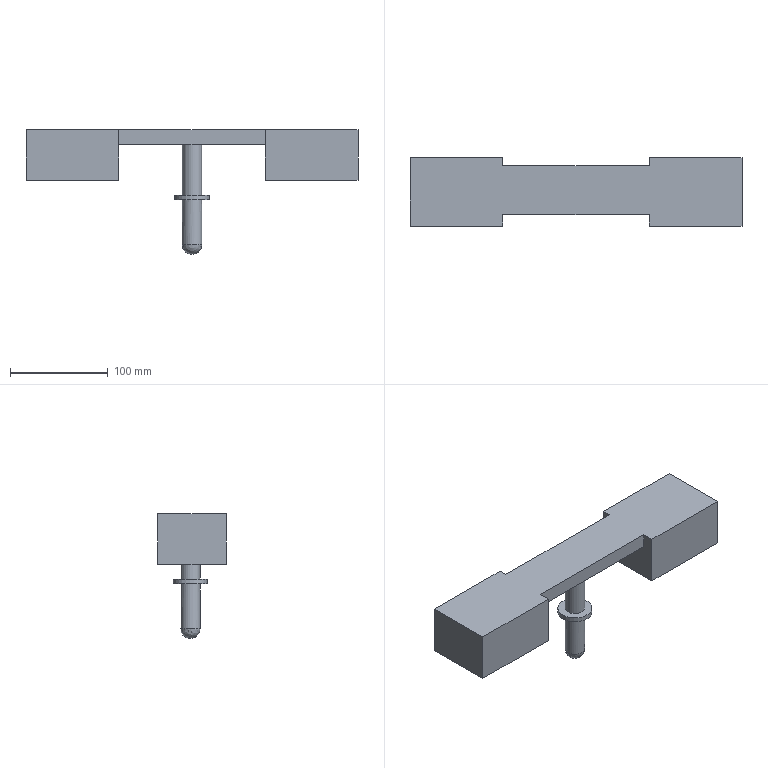Part | STEP file | tieqiantou | 1 solid | 20 faces | box 340 x 70 x 128 mm | volume 841793 mm3 | plane 16 | cylinder 3 | sphere 1 | commonest cylinder face diameters 20 x2 35 x1
STEP:
#1=CARTESIAN_POINT('',(0.,0.,0.));
#2=DIRECTION('',(0.,0.,1.));
#3=DIRECTION('',(1.,0.,0.));
#4=AXIS2_PLACEMENT_3D('',#1,#2,#3);
#5=CARTESIAN_POINT('',(-10.,0.,113.));
#6=VERTEX_POINT('',#5);
#7=CARTESIAN_POINT('',(10.,0.,113.));
#8=VERTEX_POINT('',#7);
#9=CARTESIAN_POINT('',(0.,0.,113.));
#10=DIRECTION('',(0.,0.,1.));
#11=DIRECTION('',(1.,0.,0.));
#12=AXIS2_PLACEMENT_3D('',#9,#10,#11);
#13=CIRCLE('',#12,10.);
#14=CARTESIAN_POINT('',(0.,0.,113.));
#15=DIRECTION('',(0.,0.,-1.));
#16=DIRECTION('',(-1.,0.,0.));
#17=AXIS2_PLACEMENT_3D('',#14,#15,#16);
#18=CYLINDRICAL_SURFACE('',#17,10.);
#19=CARTESIAN_POINT('',(9.425,0.));
#20=DIRECTION('',(-1.,0.));
#21=VECTOR('',#20,1.);
#22=LINE('',#19,#21);
#23=(GEOMETRIC_REPRESENTATION_CONTEXT(2)PARAMETRIC_REPRESENTATION_CONTEXT()REPRESENTATION_CONTEXT('',''));
#24=DEFINITIONAL_REPRESENTATION('',(#22),#23);
#25=PCURVE('',#18,#24);
#26=CARTESIAN_POINT('',(0.,0.,113.));
#27=DIRECTION('',(0.,0.,1.));
#28=DIRECTION('',(1.,0.,0.));
#29=AXIS2_PLACEMENT_3D('',#26,#27,#28);
#30=PLANE('',#29);
#31=CARTESIAN_POINT('',(0.,0.));
#32=DIRECTION('',(1.,0.));
#33=AXIS2_PLACEMENT_2D('',#31,#32);
#34=CIRCLE('',#33,10.);
#35=(GEOMETRIC_REPRESENTATION_CONTEXT(2)PARAMETRIC_REPRESENTATION_CONTEXT()REPRESENTATION_CONTEXT('',''));
#36=DEFINITIONAL_REPRESENTATION('',(#34),#35);
#37=PCURVE('',#30,#36);
#38=SURFACE_CURVE('',#13,(#25,#37),.PCURVE_S1.);
#39=EDGE_CURVE('',#6,#8,#38,.T.);
#40=ORIENTED_EDGE('',*,*,#39,.F.);
#41=CARTESIAN_POINT('',(-10.,0.,61.));
#42=VERTEX_POINT('',#41);
#43=CARTESIAN_POINT('',(-10.,0.,113.));
#44=CARTESIAN_POINT('',(-10.,0.,61.));
#45=B_SPLINE_CURVE_WITH_KNOTS('',1,(#43,#44),.UNSPECIFIED.,.F.,.F.,(2,2),(0.,52.),.PIECEWISE_BEZIER_KNOTS.);
#46=CARTESIAN_POINT('',(6.283,0.));
#47=DIRECTION('',(0.,1.));
#48=VECTOR('',#47,1.);
#49=LINE('',#46,#48);
#50=(GEOMETRIC_REPRESENTATION_CONTEXT(2)PARAMETRIC_REPRESENTATION_CONTEXT()REPRESENTATION_CONTEXT('',''));
#51=DEFINITIONAL_REPRESENTATION('',(#49),#50);
#52=PCURVE('',#18,#51);
#53=CARTESIAN_POINT('',(0.,0.));
#54=DIRECTION('',(0.,1.));
#55=VECTOR('',#54,1.);
#56=LINE('',#53,#55);
#57=(GEOMETRIC_REPRESENTATION_CONTEXT(2)PARAMETRIC_REPRESENTATION_CONTEXT()REPRESENTATION_CONTEXT('',''));
#58=DEFINITIONAL_REPRESENTATION('',(#56),#57);
#59=PCURVE('',#18,#58);
#60=SEAM_CURVE('',#45,(#52,#59),.PCURVE_S1.);
#61=EDGE_CURVE('',#6,#42,#60,.T.);
#62=ORIENTED_EDGE('',*,*,#61,.T.);
#63=CARTESIAN_POINT('',(0.,0.,61.));
#64=DIRECTION('',(0.,0.,-1.));
#65=DIRECTION('',(-1.,0.,0.));
#66=AXIS2_PLACEMENT_3D('',#63,#64,#65);
#67=CIRCLE('',#66,10.);
#68=CARTESIAN_POINT('',(0.,52.));
#69=DIRECTION('',(1.,0.));
#70=VECTOR('',#69,1.);
#71=LINE('',#68,#70);
#72=(GEOMETRIC_REPRESENTATION_CONTEXT(2)PARAMETRIC_REPRESENTATION_CONTEXT()REPRESENTATION_CONTEXT('',''));
#73=DEFINITIONAL_REPRESENTATION('',(#71),#72);
#74=PCURVE('',#18,#73);
#75=CARTESIAN_POINT('',(0.,0.,61.));
#76=DIRECTION('',(0.,0.,-1.));
#77=DIRECTION('',(-1.,0.,0.));
#78=AXIS2_PLACEMENT_3D('',#75,#76,#77);
#79=PLANE('',#78);
#80=CARTESIAN_POINT('',(0.,0.));
#81=DIRECTION('',(1.,0.));
#82=AXIS2_PLACEMENT_2D('',#80,#81);
#83=CIRCLE('',#82,10.);
#84=(GEOMETRIC_REPRESENTATION_CONTEXT(2)PARAMETRIC_REPRESENTATION_CONTEXT()REPRESENTATION_CONTEXT('',''));
#85=DEFINITIONAL_REPRESENTATION('',(#83),#84);
#86=PCURVE('',#79,#85);
#87=SURFACE_CURVE('',#67,(#74,#86),.PCURVE_S1.);
#88=EDGE_CURVE('',#42,#42,#87,.T.);
#89=ORIENTED_EDGE('',*,*,#88,.F.);
#90=ORIENTED_EDGE('',*,*,#61,.F.);
#91=CARTESIAN_POINT('',(0.,0.,113.));
#92=DIRECTION('',(0.,0.,1.));
#93=DIRECTION('',(1.,0.,0.));
#94=AXIS2_PLACEMENT_3D('',#91,#92,#93);
#95=CIRCLE('',#94,10.);
#96=CARTESIAN_POINT('',(3.142,0.));
#97=DIRECTION('',(-1.,0.));
#98=VECTOR('',#97,1.);
#99=LINE('',#96,#98);
#100=(GEOMETRIC_REPRESENTATION_CONTEXT(2)PARAMETRIC_REPRESENTATION_CONTEXT()REPRESENTATION_CONTEXT('',''));
#101=DEFINITIONAL_REPRESENTATION('',(#99),#100);
#102=PCURVE('',#18,#101);
#103=CARTESIAN_POINT('',(0.,0.));
#104=DIRECTION('',(1.,0.));
#105=AXIS2_PLACEMENT_2D('',#103,#104);
#106=CIRCLE('',#105,10.);
#107=(GEOMETRIC_REPRESENTATION_CONTEXT(2)PARAMETRIC_REPRESENTATION_CONTEXT()REPRESENTATION_CONTEXT('',''));
#108=DEFINITIONAL_REPRESENTATION('',(#106),#107);
#109=PCURVE('',#30,#108);
#110=SURFACE_CURVE('',#95,(#102,#109),.PCURVE_S1.);
#111=EDGE_CURVE('',#8,#6,#110,.T.);
#112=ORIENTED_EDGE('',*,*,#111,.F.);
#113=EDGE_LOOP('',(#40,#62,#89,#90,#112));
#114=FACE_BOUND('',#113,.T.);
#115=ADVANCED_FACE('',(#114),#18,.T.);
#116=ORIENTED_EDGE('',*,*,#111,.T.);
#117=ORIENTED_EDGE('',*,*,#39,.T.);
#118=EDGE_LOOP('',(#116,#117));
#119=FACE_BOUND('',#118,.T.);
#120=CARTESIAN_POINT('',(75.,-25.,113.));
#121=VERTEX_POINT('',#120);
#122=CARTESIAN_POINT('',(75.,25.,113.));
#123=VERTEX_POINT('',#122);
#124=CARTESIAN_POINT('',(75.,25.,113.));
#125=DIRECTION('',(0.,1.,0.));
#126=VECTOR('',#125,1.);
#127=LINE('',#124,#126);
#128=CARTESIAN_POINT('',(75.,25.));
#129=DIRECTION('',(0.,1.));
#130=VECTOR('',#129,1.);
#131=LINE('',#128,#130);
#132=(GEOMETRIC_REPRESENTATION_CONTEXT(2)PARAMETRIC_REPRESENTATION_CONTEXT()REPRESENTATION_CONTEXT('',''));
#133=DEFINITIONAL_REPRESENTATION('',(#131),#132);
#134=PCURVE('',#30,#133);
#135=CARTESIAN_POINT('',(75.,33.294,76.));
#136=DIRECTION('',(1.,0.,0.));
#137=DIRECTION('',(0.,1.,0.));
#138=AXIS2_PLACEMENT_3D('',#135,#136,#137);
#139=PLANE('',#138);
#140=CARTESIAN_POINT('',(-8.294,37.));
#141=DIRECTION('',(1.,0.));
#142=VECTOR('',#141,1.);
#143=LINE('',#140,#142);
#144=(GEOMETRIC_REPRESENTATION_CONTEXT(2)PARAMETRIC_REPRESENTATION_CONTEXT()REPRESENTATION_CONTEXT('',''));
#145=DEFINITIONAL_REPRESENTATION('',(#143),#144);
#146=PCURVE('',#139,#145);
#147=SURFACE_CURVE('',#127,(#134,#146),.PCURVE_S1.);
#148=EDGE_CURVE('',#121,#123,#147,.T.);
#149=ORIENTED_EDGE('',*,*,#148,.F.);
#150=CARTESIAN_POINT('',(-75.,-25.,113.));
#151=VERTEX_POINT('',#150);
#152=CARTESIAN_POINT('',(-75.,-25.,113.));
#153=DIRECTION('',(1.,0.,0.));
#154=VECTOR('',#153,1.);
#155=LINE('',#152,#154);
#156=CARTESIAN_POINT('',(-75.,-25.));
#157=DIRECTION('',(1.,0.));
#158=VECTOR('',#157,1.);
#159=LINE('',#156,#158);
#160=(GEOMETRIC_REPRESENTATION_CONTEXT(2)PARAMETRIC_REPRESENTATION_CONTEXT()REPRESENTATION_CONTEXT('',''));
#161=DEFINITIONAL_REPRESENTATION('',(#159),#160);
#162=PCURVE('',#30,#161);
#163=CARTESIAN_POINT('',(-75.,-25.,113.));
#164=DIRECTION('',(0.,-1.,0.));
#165=DIRECTION('',(0.,0.,-1.));
#166=AXIS2_PLACEMENT_3D('',#163,#164,#165);
#167=PLANE('',#166);
#168=CARTESIAN_POINT('',(0.,0.));
#169=DIRECTION('',(0.,1.));
#170=VECTOR('',#169,1.);
#171=LINE('',#168,#170);
#172=(GEOMETRIC_REPRESENTATION_CONTEXT(2)PARAMETRIC_REPRESENTATION_CONTEXT()REPRESENTATION_CONTEXT('',''));
#173=DEFINITIONAL_REPRESENTATION('',(#171),#172);
#174=PCURVE('',#167,#173);
#175=SURFACE_CURVE('',#155,(#162,#174),.PCURVE_S1.);
#176=EDGE_CURVE('',#151,#121,#175,.T.);
#177=ORIENTED_EDGE('',*,*,#176,.F.);
#178=CARTESIAN_POINT('',(-75.,25.,113.));
#179=VERTEX_POINT('',#178);
#180=CARTESIAN_POINT('',(-75.,25.,113.));
#181=DIRECTION('',(0.,-1.,0.));
#182=VECTOR('',#181,1.);
#183=LINE('',#180,#182);
#184=CARTESIAN_POINT('',(-75.,25.));
#185=DIRECTION('',(0.,-1.));
#186=VECTOR('',#185,1.);
#187=LINE('',#184,#186);
#188=(GEOMETRIC_REPRESENTATION_CONTEXT(2)PARAMETRIC_REPRESENTATION_CONTEXT()REPRESENTATION_CONTEXT('',''));
#189=DEFINITIONAL_REPRESENTATION('',(#187),#188);
#190=PCURVE('',#30,#189);
#191=CARTESIAN_POINT('',(-75.,33.294,76.));
#192=DIRECTION('',(-1.,0.,0.));
#193=DIRECTION('',(0.,-1.,0.));
#194=AXIS2_PLACEMENT_3D('',#191,#192,#193);
#195=PLANE('',#194);
#196=CARTESIAN_POINT('',(8.294,37.));
#197=DIRECTION('',(1.,0.));
#198=VECTOR('',#197,1.);
#199=LINE('',#196,#198);
#200=(GEOMETRIC_REPRESENTATION_CONTEXT(2)PARAMETRIC_REPRESENTATION_CONTEXT()REPRESENTATION_CONTEXT('',''));
#201=DEFINITIONAL_REPRESENTATION('',(#199),#200);
#202=PCURVE('',#195,#201);
#203=SURFACE_CURVE('',#183,(#190,#202),.PCURVE_S1.);
#204=EDGE_CURVE('',#179,#151,#203,.T.);
#205=ORIENTED_EDGE('',*,*,#204,.F.);
#206=CARTESIAN_POINT('',(-75.,25.,113.));
#207=DIRECTION('',(-1.,0.,0.));
#208=VECTOR('',#207,1.);
#209=LINE('',#206,#208);
#210=CARTESIAN_POINT('',(-75.,25.));
#211=DIRECTION('',(-1.,0.));
#212=VECTOR('',#211,1.);
#213=LINE('',#210,#212);
#214=(GEOMETRIC_REPRESENTATION_CONTEXT(2)PARAMETRIC_REPRESENTATION_CONTEXT()REPRESENTATION_CONTEXT('',''));
#215=DEFINITIONAL_REPRESENTATION('',(#213),#214);
#216=PCURVE('',#30,#215);
#217=CARTESIAN_POINT('',(-75.,25.,113.));
#218=DIRECTION('',(0.,1.,0.));
#219=DIRECTION('',(0.,0.,1.));
#220=AXIS2_PLACEMENT_3D('',#217,#218,#219);
#221=PLANE('',#220);
#222=CARTESIAN_POINT('',(0.,0.));
#223=DIRECTION('',(0.,-1.));
#224=VECTOR('',#223,1.);
#225=LINE('',#222,#224);
#226=(GEOMETRIC_REPRESENTATION_CONTEXT(2)PARAMETRIC_REPRESENTATION_CONTEXT()REPRESENTATION_CONTEXT('',''));
#227=DEFINITIONAL_REPRESENTATION('',(#225),#226);
#228=PCURVE('',#221,#227);
#229=SURFACE_CURVE('',#209,(#216,#228),.PCURVE_S1.);
#230=EDGE_CURVE('',#123,#179,#229,.T.);
#231=ORIENTED_EDGE('',*,*,#230,.F.);
#232=EDGE_LOOP('',(#149,#177,#205,#231));
#233=FACE_BOUND('',#232,.T.);
#234=ADVANCED_FACE('',(#119,#233),#30,.F.);
#235=CARTESIAN_POINT('',(75.,-25.,128.));
#236=VERTEX_POINT('',#235);
#237=CARTESIAN_POINT('',(75.,-25.,113.));
#238=DIRECTION('',(0.,0.,1.));
#239=VECTOR('',#238,1.);
#240=LINE('',#237,#239);
#241=CARTESIAN_POINT('',(0.,150.));
#242=DIRECTION('',(-1.,0.));
#243=VECTOR('',#242,1.);
#244=LINE('',#241,#243);
#245=(GEOMETRIC_REPRESENTATION_CONTEXT(2)PARAMETRIC_REPRESENTATION_CONTEXT()REPRESENTATION_CONTEXT('',''));
#246=DEFINITIONAL_REPRESENTATION('',(#244),#245);
#247=PCURVE('',#167,#246);
#248=CARTESIAN_POINT('',(-58.294,37.));
#249=DIRECTION('',(0.,1.));
#250=VECTOR('',#249,1.);
#251=LINE('',#248,#250);
#252=(GEOMETRIC_REPRESENTATION_CONTEXT(2)PARAMETRIC_REPRESENTATION_CONTEXT()REPRESENTATION_CONTEXT('',''));
#253=DEFINITIONAL_REPRESENTATION('',(#251),#252);
#254=PCURVE('',#139,#253);
#255=SURFACE_CURVE('',#240,(#247,#254),.PCURVE_S1.);
#256=EDGE_CURVE('',#121,#236,#255,.T.);
#257=ORIENTED_EDGE('',*,*,#256,.T.);
#258=CARTESIAN_POINT('',(-75.,-25.,128.));
#259=VERTEX_POINT('',#258);
#260=CARTESIAN_POINT('',(-75.,-25.,128.));
#261=DIRECTION('',(1.,0.,0.));
#262=VECTOR('',#261,1.);
#263=LINE('',#260,#262);
#264=CARTESIAN_POINT('',(-15.,0.));
#265=DIRECTION('',(0.,1.));
#266=VECTOR('',#265,1.);
#267=LINE('',#264,#266);
#268=(GEOMETRIC_REPRESENTATION_CONTEXT(2)PARAMETRIC_REPRESENTATION_CONTEXT()REPRESENTATION_CONTEXT('',''));
#269=DEFINITIONAL_REPRESENTATION('',(#267),#268);
#270=PCURVE('',#167,#269);
#271=CARTESIAN_POINT('',(0.,0.,128.));
#272=DIRECTION('',(0.,0.,1.));
#273=DIRECTION('',(1.,0.,0.));
#274=AXIS2_PLACEMENT_3D('',#271,#272,#273);
#275=PLANE('',#274);
#276=CARTESIAN_POINT('',(-75.,-25.));
#277=DIRECTION('',(1.,0.));
#278=VECTOR('',#277,1.);
#279=LINE('',#276,#278);
#280=(GEOMETRIC_REPRESENTATION_CONTEXT(2)PARAMETRIC_REPRESENTATION_CONTEXT()REPRESENTATION_CONTEXT('',''));
#281=DEFINITIONAL_REPRESENTATION('',(#279),#280);
#282=PCURVE('',#275,#281);
#283=SURFACE_CURVE('',#263,(#270,#282),.PCURVE_S1.);
#284=EDGE_CURVE('',#259,#236,#283,.T.);
#285=ORIENTED_EDGE('',*,*,#284,.F.);
#286=CARTESIAN_POINT('',(-75.,-25.,113.));
#287=DIRECTION('',(0.,0.,1.));
#288=VECTOR('',#287,1.);
#289=LINE('',#286,#288);
#290=CARTESIAN_POINT('',(0.,0.));
#291=DIRECTION('',(-1.,0.));
#292=VECTOR('',#291,1.);
#293=LINE('',#290,#292);
#294=(GEOMETRIC_REPRESENTATION_CONTEXT(2)PARAMETRIC_REPRESENTATION_CONTEXT()REPRESENTATION_CONTEXT('',''));
#295=DEFINITIONAL_REPRESENTATION('',(#293),#294);
#296=PCURVE('',#167,#295);
#297=CARTESIAN_POINT('',(58.294,37.));
#298=DIRECTION('',(0.,1.));
#299=VECTOR('',#298,1.);
#300=LINE('',#297,#299);
#301=(GEOMETRIC_REPRESENTATION_CONTEXT(2)PARAMETRIC_REPRESENTATION_CONTEXT()REPRESENTATION_CONTEXT('',''));
#302=DEFINITIONAL_REPRESENTATION('',(#300),#301);
#303=PCURVE('',#195,#302);
#304=SURFACE_CURVE('',#289,(#296,#303),.PCURVE_S1.);
#305=EDGE_CURVE('',#151,#259,#304,.T.);
#306=ORIENTED_EDGE('',*,*,#305,.F.);
#307=ORIENTED_EDGE('',*,*,#176,.T.);
#308=EDGE_LOOP('',(#257,#285,#306,#307));
#309=FACE_BOUND('',#308,.T.);
#310=ADVANCED_FACE('',(#309),#167,.T.);
#311=CARTESIAN_POINT('',(-75.,25.,128.));
#312=VERTEX_POINT('',#311);
#313=CARTESIAN_POINT('',(-75.,25.,113.));
#314=DIRECTION('',(0.,0.,1.));
#315=VECTOR('',#314,1.);
#316=LINE('',#313,#315);
#317=CARTESIAN_POINT('',(0.,0.));
#318=DIRECTION('',(1.,0.));
#319=VECTOR('',#318,1.);
#320=LINE('',#317,#319);
#321=(GEOMETRIC_REPRESENTATION_CONTEXT(2)PARAMETRIC_REPRESENTATION_CONTEXT()REPRESENTATION_CONTEXT('',''));
#322=DEFINITIONAL_REPRESENTATION('',(#320),#321);
#323=PCURVE('',#221,#322);
#324=CARTESIAN_POINT('',(8.294,37.));
#325=DIRECTION('',(0.,1.));
#326=VECTOR('',#325,1.);
#327=LINE('',#324,#326);
#328=(GEOMETRIC_REPRESENTATION_CONTEXT(2)PARAMETRIC_REPRESENTATION_CONTEXT()REPRESENTATION_CONTEXT('',''));
#329=DEFINITIONAL_REPRESENTATION('',(#327),#328);
#330=PCURVE('',#195,#329);
#331=SURFACE_CURVE('',#316,(#323,#330),.PCURVE_S1.);
#332=EDGE_CURVE('',#179,#312,#331,.T.);
#333=ORIENTED_EDGE('',*,*,#332,.T.);
#334=CARTESIAN_POINT('',(75.,25.,128.));
#335=VERTEX_POINT('',#334);
#336=CARTESIAN_POINT('',(-75.,25.,128.));
#337=DIRECTION('',(-1.,0.,0.));
#338=VECTOR('',#337,1.);
#339=LINE('',#336,#338);
#340=CARTESIAN_POINT('',(15.,0.));
#341=DIRECTION('',(0.,-1.));
#342=VECTOR('',#341,1.);
#343=LINE('',#340,#342);
#344=(GEOMETRIC_REPRESENTATION_CONTEXT(2)PARAMETRIC_REPRESENTATION_CONTEXT()REPRESENTATION_CONTEXT('',''));
#345=DEFINITIONAL_REPRESENTATION('',(#343),#344);
#346=PCURVE('',#221,#345);
#347=CARTESIAN_POINT('',(-75.,25.));
#348=DIRECTION('',(-1.,0.));
#349=VECTOR('',#348,1.);
#350=LINE('',#347,#349);
#351=(GEOMETRIC_REPRESENTATION_CONTEXT(2)PARAMETRIC_REPRESENTATION_CONTEXT()REPRESENTATION_CONTEXT('',''));
#352=DEFINITIONAL_REPRESENTATION('',(#350),#351);
#353=PCURVE('',#275,#352);
#354=SURFACE_CURVE('',#339,(#346,#353),.PCURVE_S1.);
#355=EDGE_CURVE('',#335,#312,#354,.T.);
#356=ORIENTED_EDGE('',*,*,#355,.F.);
#357=CARTESIAN_POINT('',(75.,25.,113.));
#358=DIRECTION('',(0.,0.,1.));
#359=VECTOR('',#358,1.);
#360=LINE('',#357,#359);
#361=CARTESIAN_POINT('',(0.,150.));
#362=DIRECTION('',(1.,0.));
#363=VECTOR('',#362,1.);
#364=LINE('',#361,#363);
#365=(GEOMETRIC_REPRESENTATION_CONTEXT(2)PARAMETRIC_REPRESENTATION_CONTEXT()REPRESENTATION_CONTEXT('',''));
#366=DEFINITIONAL_REPRESENTATION('',(#364),#365);
#367=PCURVE('',#221,#366);
#368=CARTESIAN_POINT('',(-8.294,37.));
#369=DIRECTION('',(0.,1.));
#370=VECTOR('',#369,1.);
#371=LINE('',#368,#370);
#372=(GEOMETRIC_REPRESENTATION_CONTEXT(2)PARAMETRIC_REPRESENTATION_CONTEXT()REPRESENTATION_CONTEXT('',''));
#373=DEFINITIONAL_REPRESENTATION('',(#371),#372);
#374=PCURVE('',#139,#373);
#375=SURFACE_CURVE('',#360,(#367,#374),.PCURVE_S1.);
#376=EDGE_CURVE('',#123,#335,#375,.T.);
#377=ORIENTED_EDGE('',*,*,#376,.F.);
#378=ORIENTED_EDGE('',*,*,#230,.T.);
#379=EDGE_LOOP('',(#333,#356,#377,#378));
#380=FACE_BOUND('',#379,.T.);
#381=ADVANCED_FACE('',(#380),#221,.T.);
#382=ORIENTED_EDGE('',*,*,#284,.T.);
#383=CARTESIAN_POINT('',(75.,-36.706,128.));
#384=VERTEX_POINT('',#383);
#385=CARTESIAN_POINT('',(75.,33.294,128.));
#386=DIRECTION('',(0.,1.,0.));
#387=VECTOR('',#386,1.);
#388=LINE('',#385,#387);
#389=CARTESIAN_POINT('',(75.,33.294));
#390=DIRECTION('',(0.,1.));
#391=VECTOR('',#390,1.);
#392=LINE('',#389,#391);
#393=(GEOMETRIC_REPRESENTATION_CONTEXT(2)PARAMETRIC_REPRESENTATION_CONTEXT()REPRESENTATION_CONTEXT('',''));
#394=DEFINITIONAL_REPRESENTATION('',(#392),#393);
#395=PCURVE('',#275,#394);
#396=CARTESIAN_POINT('',(0.,52.));
#397=DIRECTION('',(1.,0.));
#398=VECTOR('',#397,1.);
#399=LINE('',#396,#398);
#400=(GEOMETRIC_REPRESENTATION_CONTEXT(2)PARAMETRIC_REPRESENTATION_CONTEXT()REPRESENTATION_CONTEXT('',''));
#401=DEFINITIONAL_REPRESENTATION('',(#399),#400);
#402=PCURVE('',#139,#401);
#403=SURFACE_CURVE('',#388,(#395,#402),.PCURVE_S1.);
#404=EDGE_CURVE('',#384,#236,#403,.T.);
#405=ORIENTED_EDGE('',*,*,#404,.F.);
#406=CARTESIAN_POINT('',(170.,-36.706,128.));
#407=VERTEX_POINT('',#406);
#408=CARTESIAN_POINT('',(170.,-36.706,128.));
#409=DIRECTION('',(-1.,0.,0.));
#410=VECTOR('',#409,1.);
#411=LINE('',#408,#410);
#412=CARTESIAN_POINT('',(170.,-36.706));
#413=DIRECTION('',(-1.,0.));
#414=VECTOR('',#413,1.);
#415=LINE('',#412,#414);
#416=(GEOMETRIC_REPRESENTATION_CONTEXT(2)PARAMETRIC_REPRESENTATION_CONTEXT()REPRESENTATION_CONTEXT('',''));
#417=DEFINITIONAL_REPRESENTATION('',(#415),#416);
#418=PCURVE('',#275,#417);
#419=CARTESIAN_POINT('',(170.,-36.706,76.));
#420=DIRECTION('',(0.,1.,0.));
#421=DIRECTION('',(-1.,0.,0.));
#422=AXIS2_PLACEMENT_3D('',#419,#420,#421);
#423=PLANE('',#422);
#424=CARTESIAN_POINT('',(0.,52.));
#425=DIRECTION('',(1.,0.));
#426=VECTOR('',#425,1.);
#427=LINE('',#424,#426);
#428=(GEOMETRIC_REPRESENTATION_CONTEXT(2)PARAMETRIC_REPRESENTATION_CONTEXT()REPRESENTATION_CONTEXT('',''));
#429=DEFINITIONAL_REPRESENTATION('',(#427),#428);
#430=PCURVE('',#423,#429);
#431=SURFACE_CURVE('',#411,(#418,#430),.PCURVE_S1.);
#432=EDGE_CURVE('',#407,#384,#431,.T.);
#433=ORIENTED_EDGE('',*,*,#432,.F.);
#434=CARTESIAN_POINT('',(170.,33.294,128.));
#435=VERTEX_POINT('',#434);
#436=CARTESIAN_POINT('',(170.,33.294,128.));
#437=DIRECTION('',(0.,-1.,0.));
#438=VECTOR('',#437,1.);
#439=LINE('',#436,#438);
#440=CARTESIAN_POINT('',(170.,33.294));
#441=DIRECTION('',(0.,-1.));
#442=VECTOR('',#441,1.);
#443=LINE('',#440,#442);
#444=(GEOMETRIC_REPRESENTATION_CONTEXT(2)PARAMETRIC_REPRESENTATION_CONTEXT()REPRESENTATION_CONTEXT('',''));
#445=DEFINITIONAL_REPRESENTATION('',(#443),#444);
#446=PCURVE('',#275,#445);
#447=CARTESIAN_POINT('',(170.,33.294,76.));
#448=DIRECTION('',(-1.,0.,0.));
#449=DIRECTION('',(0.,-1.,0.));
#450=AXIS2_PLACEMENT_3D('',#447,#448,#449);
#451=PLANE('',#450);
#452=CARTESIAN_POINT('',(0.,52.));
#453=DIRECTION('',(1.,0.));
#454=VECTOR('',#453,1.);
#455=LINE('',#452,#454);
#456=(GEOMETRIC_REPRESENTATION_CONTEXT(2)PARAMETRIC_REPRESENTATION_CONTEXT()REPRESENTATION_CONTEXT('',''));
#457=DEFINITIONAL_REPRESENTATION('',(#455),#456);
#458=PCURVE('',#451,#457);
#459=SURFACE_CURVE('',#439,(#446,#458),.PCURVE_S1.);
#460=EDGE_CURVE('',#435,#407,#459,.T.);
#461=ORIENTED_EDGE('',*,*,#460,.F.);
#462=CARTESIAN_POINT('',(75.,33.294,128.));
#463=VERTEX_POINT('',#462);
#464=CARTESIAN_POINT('',(170.,33.294,128.));
#465=DIRECTION('',(1.,0.,0.));
#466=VECTOR('',#465,1.);
#467=LINE('',#464,#466);
#468=CARTESIAN_POINT('',(170.,33.294));
#469=DIRECTION('',(1.,0.));
#470=VECTOR('',#469,1.);
#471=LINE('',#468,#470);
#472=(GEOMETRIC_REPRESENTATION_CONTEXT(2)PARAMETRIC_REPRESENTATION_CONTEXT()REPRESENTATION_CONTEXT('',''));
#473=DEFINITIONAL_REPRESENTATION('',(#471),#472);
#474=PCURVE('',#275,#473);
#475=CARTESIAN_POINT('',(170.,33.294,76.));
#476=DIRECTION('',(0.,-1.,0.));
#477=DIRECTION('',(1.,0.,0.));
#478=AXIS2_PLACEMENT_3D('',#475,#476,#477);
#479=PLANE('',#478);
#480=CARTESIAN_POINT('',(0.,52.));
#481=DIRECTION('',(1.,0.));
#482=VECTOR('',#481,1.);
#483=LINE('',#480,#482);
#484=(GEOMETRIC_REPRESENTATION_CONTEXT(2)PARAMETRIC_REPRESENTATION_CONTEXT()REPRESENTATION_CONTEXT('',''));
#485=DEFINITIONAL_REPRESENTATION('',(#483),#484);
#486=PCURVE('',#479,#485);
#487=SURFACE_CURVE('',#467,(#474,#486),.PCURVE_S1.);
#488=EDGE_CURVE('',#463,#435,#487,.T.);
#489=ORIENTED_EDGE('',*,*,#488,.F.);
#490=CARTESIAN_POINT('',(75.,33.294,128.));
#491=DIRECTION('',(0.,1.,0.));
#492=VECTOR('',#491,1.);
#493=LINE('',#490,#492);
#494=CARTESIAN_POINT('',(75.,33.294));
#495=DIRECTION('',(0.,1.));
#496=VECTOR('',#495,1.);
#497=LINE('',#494,#496);
#498=(GEOMETRIC_REPRESENTATION_CONTEXT(2)PARAMETRIC_REPRESENTATION_CONTEXT()REPRESENTATION_CONTEXT('',''));
#499=DEFINITIONAL_REPRESENTATION('',(#497),#498);
#500=PCURVE('',#275,#499);
#501=CARTESIAN_POINT('',(0.,52.));
#502=DIRECTION('',(1.,0.));
#503=VECTOR('',#502,1.);
#504=LINE('',#501,#503);
#505=(GEOMETRIC_REPRESENTATION_CONTEXT(2)PARAMETRIC_REPRESENTATION_CONTEXT()REPRESENTATION_CONTEXT('',''));
#506=DEFINITIONAL_REPRESENTATION('',(#504),#505);
#507=PCURVE('',#139,#506);
#508=SURFACE_CURVE('',#493,(#500,#507),.PCURVE_S1.);
#509=EDGE_CURVE('',#335,#463,#508,.T.);
#510=ORIENTED_EDGE('',*,*,#509,.F.);
#511=ORIENTED_EDGE('',*,*,#355,.T.);
#512=CARTESIAN_POINT('',(-75.,33.294,128.));
#513=VERTEX_POINT('',#512);
#514=CARTESIAN_POINT('',(-75.,33.294,128.));
#515=DIRECTION('',(0.,-1.,0.));
#516=VECTOR('',#515,1.);
#517=LINE('',#514,#516);
#518=CARTESIAN_POINT('',(-75.,33.294));
#519=DIRECTION('',(0.,-1.));
#520=VECTOR('',#519,1.);
#521=LINE('',#518,#520);
#522=(GEOMETRIC_REPRESENTATION_CONTEXT(2)PARAMETRIC_REPRESENTATION_CONTEXT()REPRESENTATION_CONTEXT('',''));
#523=DEFINITIONAL_REPRESENTATION('',(#521),#522);
#524=PCURVE('',#275,#523);
#525=CARTESIAN_POINT('',(0.,52.));
#526=DIRECTION('',(1.,0.));
#527=VECTOR('',#526,1.);
#528=LINE('',#525,#527);
#529=(GEOMETRIC_REPRESENTATION_CONTEXT(2)PARAMETRIC_REPRESENTATION_CONTEXT()REPRESENTATION_CONTEXT('',''));
#530=DEFINITIONAL_REPRESENTATION('',(#528),#529);
#531=PCURVE('',#195,#530);
#532=SURFACE_CURVE('',#517,(#524,#531),.PCURVE_S1.);
#533=EDGE_CURVE('',#513,#312,#532,.T.);
#534=ORIENTED_EDGE('',*,*,#533,.F.);
#535=CARTESIAN_POINT('',(-170.,33.294,128.));
#536=VERTEX_POINT('',#535);
#537=CARTESIAN_POINT('',(-170.,33.294,128.));
#538=DIRECTION('',(1.,0.,0.));
#539=VECTOR('',#538,1.);
#540=LINE('',#537,#539);
#541=CARTESIAN_POINT('',(-170.,33.294));
#542=DIRECTION('',(1.,0.));
#543=VECTOR('',#542,1.);
#544=LINE('',#541,#543);
#545=(GEOMETRIC_REPRESENTATION_CONTEXT(2)PARAMETRIC_REPRESENTATION_CONTEXT()REPRESENTATION_CONTEXT('',''));
#546=DEFINITIONAL_REPRESENTATION('',(#544),#545);
#547=PCURVE('',#275,#546);
#548=CARTESIAN_POINT('',(-170.,33.294,76.));
#549=DIRECTION('',(0.,-1.,0.));
#550=DIRECTION('',(1.,0.,0.));
#551=AXIS2_PLACEMENT_3D('',#548,#549,#550);
#552=PLANE('',#551);
#553=CARTESIAN_POINT('',(0.,52.));
#554=DIRECTION('',(1.,0.));
#555=VECTOR('',#554,1.);
#556=LINE('',#553,#555);
#557=(GEOMETRIC_REPRESENTATION_CONTEXT(2)PARAMETRIC_REPRESENTATION_CONTEXT()REPRESENTATION_CONTEXT('',''));
#558=DEFINITIONAL_REPRESENTATION('',(#556),#557);
#559=PCURVE('',#552,#558);
#560=SURFACE_CURVE('',#540,(#547,#559),.PCURVE_S1.);
#561=EDGE_CURVE('',#536,#513,#560,.T.);
#562=ORIENTED_EDGE('',*,*,#561,.F.);
#563=CARTESIAN_POINT('',(-170.,-36.706,128.));
#564=VERTEX_POINT('',#563);
#565=CARTESIAN_POINT('',(-170.,33.294,128.));
#566=DIRECTION('',(0.,1.,0.));
#567=VECTOR('',#566,1.);
#568=LINE('',#565,#567);
#569=CARTESIAN_POINT('',(-170.,33.294));
#570=DIRECTION('',(0.,1.));
#571=VECTOR('',#570,1.);
#572=LINE('',#569,#571);
#573=(GEOMETRIC_REPRESENTATION_CONTEXT(2)PARAMETRIC_REPRESENTATION_CONTEXT()REPRESENTATION_CONTEXT('',''));
#574=DEFINITIONAL_REPRESENTATION('',(#572),#573);
#575=PCURVE('',#275,#574);
#576=CARTESIAN_POINT('',(-170.,33.294,76.));
#577=DIRECTION('',(1.,0.,0.));
#578=DIRECTION('',(0.,1.,0.));
#579=AXIS2_PLACEMENT_3D('',#576,#577,#578);
#580=PLANE('',#579);
#581=CARTESIAN_POINT('',(0.,52.));
#582=DIRECTION('',(1.,0.));
#583=VECTOR('',#582,1.);
#584=LINE('',#581,#583);
#585=(GEOMETRIC_REPRESENTATION_CONTEXT(2)PARAMETRIC_REPRESENTATION_CONTEXT()REPRESENTATION_CONTEXT('',''));
#586=DEFINITIONAL_REPRESENTATION('',(#584),#585);
#587=PCURVE('',#580,#586);
#588=SURFACE_CURVE('',#568,(#575,#587),.PCURVE_S1.);
#589=EDGE_CURVE('',#564,#536,#588,.T.);
#590=ORIENTED_EDGE('',*,*,#589,.F.);
#591=CARTESIAN_POINT('',(-75.,-36.706,128.));
#592=VERTEX_POINT('',#591);
#593=CARTESIAN_POINT('',(-170.,-36.706,128.));
#594=DIRECTION('',(-1.,0.,0.));
#595=VECTOR('',#594,1.);
#596=LINE('',#593,#595);
#597=CARTESIAN_POINT('',(-170.,-36.706));
#598=DIRECTION('',(-1.,0.));
#599=VECTOR('',#598,1.);
#600=LINE('',#597,#599);
#601=(GEOMETRIC_REPRESENTATION_CONTEXT(2)PARAMETRIC_REPRESENTATION_CONTEXT()REPRESENTATION_CONTEXT('',''));
#602=DEFINITIONAL_REPRESENTATION('',(#600),#601);
#603=PCURVE('',#275,#602);
#604=CARTESIAN_POINT('',(-170.,-36.706,76.));
#605=DIRECTION('',(0.,1.,0.));
#606=DIRECTION('',(-1.,0.,0.));
#607=AXIS2_PLACEMENT_3D('',#604,#605,#606);
#608=PLANE('',#607);
#609=CARTESIAN_POINT('',(0.,52.));
#610=DIRECTION('',(1.,0.));
#611=VECTOR('',#610,1.);
#612=LINE('',#609,#611);
#613=(GEOMETRIC_REPRESENTATION_CONTEXT(2)PARAMETRIC_REPRESENTATION_CONTEXT()REPRESENTATION_CONTEXT('',''));
#614=DEFINITIONAL_REPRESENTATION('',(#612),#613);
#615=PCURVE('',#608,#614);
#616=SURFACE_CURVE('',#596,(#603,#615),.PCURVE_S1.);
#617=EDGE_CURVE('',#592,#564,#616,.T.);
#618=ORIENTED_EDGE('',*,*,#617,.F.);
#619=CARTESIAN_POINT('',(-75.,33.294,128.));
#620=DIRECTION('',(0.,-1.,0.));
#621=VECTOR('',#620,1.);
#622=LINE('',#619,#621);
#623=CARTESIAN_POINT('',(-75.,33.294));
#624=DIRECTION('',(0.,-1.));
#625=VECTOR('',#624,1.);
#626=LINE('',#623,#625);
#627=(GEOMETRIC_REPRESENTATION_CONTEXT(2)PARAMETRIC_REPRESENTATION_CONTEXT()REPRESENTATION_CONTEXT('',''));
#628=DEFINITIONAL_REPRESENTATION('',(#626),#627);
#629=PCURVE('',#275,#628);
#630=CARTESIAN_POINT('',(0.,52.));
#631=DIRECTION('',(1.,0.));
#632=VECTOR('',#631,1.);
#633=LINE('',#630,#632);
#634=(GEOMETRIC_REPRESENTATION_CONTEXT(2)PARAMETRIC_REPRESENTATION_CONTEXT()REPRESENTATION_CONTEXT('',''));
#635=DEFINITIONAL_REPRESENTATION('',(#633),#634);
#636=PCURVE('',#195,#635);
#637=SURFACE_CURVE('',#622,(#629,#636),.PCURVE_S1.);
#638=EDGE_CURVE('',#259,#592,#637,.T.);
#639=ORIENTED_EDGE('',*,*,#638,.F.);
#640=EDGE_LOOP('',(#382,#405,#433,#461,#489,#510,#511,#534,#562,#590,#618,#639));
#641=FACE_BOUND('',#640,.T.);
#642=ADVANCED_FACE('',(#641),#275,.T.);
#643=CARTESIAN_POINT('',(-17.5,0.,56.));
#644=VERTEX_POINT('',#643);
#645=CARTESIAN_POINT('',(0.,0.,56.));
#646=DIRECTION('',(0.,0.,-1.));
#647=DIRECTION('',(-1.,0.,0.));
#648=AXIS2_PLACEMENT_3D('',#645,#646,#647);
#649=CIRCLE('',#648,17.5);
#650=CARTESIAN_POINT('',(0.,0.,56.));
#651=DIRECTION('',(0.,0.,1.));
#652=DIRECTION('',(1.,0.,0.));
#653=AXIS2_PLACEMENT_3D('',#650,#651,#652);
#654=CYLINDRICAL_SURFACE('',#653,17.5);
#655=CARTESIAN_POINT('',(9.425,0.));
#656=DIRECTION('',(-1.,0.));
#657=VECTOR('',#656,1.);
#658=LINE('',#655,#657);
#659=(GEOMETRIC_REPRESENTATION_CONTEXT(2)PARAMETRIC_REPRESENTATION_CONTEXT()REPRESENTATION_CONTEXT('',''));
#660=DEFINITIONAL_REPRESENTATION('',(#658),#659);
#661=PCURVE('',#654,#660);
#662=CARTESIAN_POINT('',(0.,0.,56.));
#663=DIRECTION('',(0.,0.,-1.));
#664=DIRECTION('',(-1.,0.,0.));
#665=AXIS2_PLACEMENT_3D('',#662,#663,#664);
#666=PLANE('',#665);
#667=CARTESIAN_POINT('',(0.,0.));
#668=DIRECTION('',(1.,0.));
#669=AXIS2_PLACEMENT_2D('',#667,#668);
#670=CIRCLE('',#669,17.5);
#671=(GEOMETRIC_REPRESENTATION_CONTEXT(2)PARAMETRIC_REPRESENTATION_CONTEXT()REPRESENTATION_CONTEXT('',''));
#672=DEFINITIONAL_REPRESENTATION('',(#670),#671);
#673=PCURVE('',#666,#672);
#674=SURFACE_CURVE('',#649,(#661,#673),.PCURVE_S1.);
#675=EDGE_CURVE('',#644,#644,#674,.T.);
#676=ORIENTED_EDGE('',*,*,#675,.F.);
#677=CARTESIAN_POINT('',(-17.5,0.,61.));
#678=VERTEX_POINT('',#677);
#679=CARTESIAN_POINT('',(-17.5,0.,56.));
#680=CARTESIAN_POINT('',(-17.5,0.,61.));
#681=B_SPLINE_CURVE_WITH_KNOTS('',1,(#679,#680),.UNSPECIFIED.,.F.,.F.,(2,2),(0.,5.),.PIECEWISE_BEZIER_KNOTS.);
#682=CARTESIAN_POINT('',(9.425,0.));
#683=DIRECTION('',(0.,1.));
#684=VECTOR('',#683,1.);
#685=LINE('',#682,#684);
#686=(GEOMETRIC_REPRESENTATION_CONTEXT(2)PARAMETRIC_REPRESENTATION_CONTEXT()REPRESENTATION_CONTEXT('',''));
#687=DEFINITIONAL_REPRESENTATION('',(#685),#686);
#688=PCURVE('',#654,#687);
#689=CARTESIAN_POINT('',(3.142,0.));
#690=DIRECTION('',(0.,1.));
#691=VECTOR('',#690,1.);
#692=LINE('',#689,#691);
#693=(GEOMETRIC_REPRESENTATION_CONTEXT(2)PARAMETRIC_REPRESENTATION_CONTEXT()REPRESENTATION_CONTEXT('',''));
#694=DEFINITIONAL_REPRESENTATION('',(#692),#693);
#695=PCURVE('',#654,#694);
#696=SEAM_CURVE('',#681,(#688,#695),.PCURVE_S1.);
#697=EDGE_CURVE('',#644,#678,#696,.T.);
#698=ORIENTED_EDGE('',*,*,#697,.T.);
#699=CARTESIAN_POINT('',(0.,0.,61.));
#700=DIRECTION('',(0.,0.,-1.));
#701=DIRECTION('',(-1.,0.,0.));
#702=AXIS2_PLACEMENT_3D('',#699,#700,#701);
#703=CIRCLE('',#702,17.5);
#704=CARTESIAN_POINT('',(9.425,5.));
#705=DIRECTION('',(-1.,0.));
#706=VECTOR('',#705,1.);
#707=LINE('',#704,#706);
#708=(GEOMETRIC_REPRESENTATION_CONTEXT(2)PARAMETRIC_REPRESENTATION_CONTEXT()REPRESENTATION_CONTEXT('',''));
#709=DEFINITIONAL_REPRESENTATION('',(#707),#708);
#710=PCURVE('',#654,#709);
#711=CARTESIAN_POINT('',(0.,0.));
#712=DIRECTION('',(1.,0.));
#713=AXIS2_PLACEMENT_2D('',#711,#712);
#714=CIRCLE('',#713,17.5);
#715=(GEOMETRIC_REPRESENTATION_CONTEXT(2)PARAMETRIC_REPRESENTATION_CONTEXT()REPRESENTATION_CONTEXT('',''));
#716=DEFINITIONAL_REPRESENTATION('',(#714),#715);
#717=PCURVE('',#79,#716);
#718=SURFACE_CURVE('',#703,(#710,#717),.PCURVE_S1.);
#719=EDGE_CURVE('',#678,#678,#718,.T.);
#720=ORIENTED_EDGE('',*,*,#719,.T.);
#721=ORIENTED_EDGE('',*,*,#697,.F.);
#722=EDGE_LOOP('',(#676,#698,#720,#721));
#723=FACE_BOUND('',#722,.T.);
#724=ADVANCED_FACE('',(#723),#654,.T.);
#725=CARTESIAN_POINT('',(-10.,0.,56.));
#726=VERTEX_POINT('',#725);
#727=CARTESIAN_POINT('',(0.,0.,56.));
#728=DIRECTION('',(0.,0.,-1.));
#729=DIRECTION('',(-1.,0.,0.));
#730=AXIS2_PLACEMENT_3D('',#727,#728,#729);
#731=CIRCLE('',#730,10.);
#732=CARTESIAN_POINT('',(0.,0.));
#733=DIRECTION('',(1.,0.));
#734=AXIS2_PLACEMENT_2D('',#732,#733);
#735=CIRCLE('',#734,10.);
#736=(GEOMETRIC_REPRESENTATION_CONTEXT(2)PARAMETRIC_REPRESENTATION_CONTEXT()REPRESENTATION_CONTEXT('',''));
#737=DEFINITIONAL_REPRESENTATION('',(#735),#736);
#738=PCURVE('',#666,#737);
#739=CARTESIAN_POINT('',(0.,0.,113.));
#740=DIRECTION('',(0.,0.,-1.));
#741=DIRECTION('',(-1.,0.,0.));
#742=AXIS2_PLACEMENT_3D('',#739,#740,#741);
#743=CYLINDRICAL_SURFACE('',#742,10.);
#744=CARTESIAN_POINT('',(0.,57.));
#745=DIRECTION('',(1.,0.));
#746=VECTOR('',#745,1.);
#747=LINE('',#744,#746);
#748=(GEOMETRIC_REPRESENTATION_CONTEXT(2)PARAMETRIC_REPRESENTATION_CONTEXT()REPRESENTATION_CONTEXT('',''));
#749=DEFINITIONAL_REPRESENTATION('',(#747),#748);
#750=PCURVE('',#743,#749);
#751=SURFACE_CURVE('',#731,(#738,#750),.PCURVE_S1.);
#752=EDGE_CURVE('',#726,#726,#751,.T.);
#753=ORIENTED_EDGE('',*,*,#752,.F.);
#754=EDGE_LOOP('',(#753));
#755=FACE_BOUND('',#754,.T.);
#756=ORIENTED_EDGE('',*,*,#675,.T.);
#757=EDGE_LOOP('',(#756));
#758=FACE_BOUND('',#757,.T.);
#759=ADVANCED_FACE('',(#755,#758),#666,.T.);
#760=ORIENTED_EDGE('',*,*,#88,.T.);
#761=EDGE_LOOP('',(#760));
#762=FACE_BOUND('',#761,.T.);
#763=ORIENTED_EDGE('',*,*,#719,.F.);
#764=EDGE_LOOP('',(#763));
#765=FACE_BOUND('',#764,.T.);
#766=ADVANCED_FACE('',(#762,#765),#79,.F.);
#767=CARTESIAN_POINT('',(0.,10.,10.));
#768=VERTEX_POINT('',#767);
#769=CARTESIAN_POINT('',(-10.,0.,10.));
#770=VERTEX_POINT('',#769);
#771=CARTESIAN_POINT('',(0.,0.,10.));
#772=DIRECTION('',(0.,0.,1.));
#773=DIRECTION('',(-1.,0.,0.));
#774=AXIS2_PLACEMENT_3D('',#771,#772,#773);
#775=CIRCLE('',#774,10.);
#776=CARTESIAN_POINT('',(0.,0.,10.));
#777=DIRECTION('',(0.,1.,0.));
#778=DIRECTION('',(1.,0.,0.));
#779=AXIS2_PLACEMENT_3D('',#776,#777,#778);
#780=SPHERICAL_SURFACE('',#779,10.);
#781=CARTESIAN_POINT('',(3.142,1.571));
#782=CARTESIAN_POINT('',(3.142,1.547));
#783=CARTESIAN_POINT('',(3.142,1.499));
#784=CARTESIAN_POINT('',(3.142,1.428));
#785=CARTESIAN_POINT('',(3.142,1.357));
#786=CARTESIAN_POINT('',(3.142,1.285));
#787=CARTESIAN_POINT('',(3.142,1.214));
#788=CARTESIAN_POINT('',(3.142,1.142));
#789=CARTESIAN_POINT('',(3.142,1.071));
#790=CARTESIAN_POINT('',(3.142,0.9996));
#791=CARTESIAN_POINT('',(3.142,0.9282));
#792=CARTESIAN_POINT('',(3.142,0.8568));
#793=CARTESIAN_POINT('',(3.142,0.7854));
#794=CARTESIAN_POINT('',(3.142,0.714));
#795=CARTESIAN_POINT('',(3.142,0.6426));
#796=CARTESIAN_POINT('',(3.142,0.5712));
#797=CARTESIAN_POINT('',(3.142,0.4998));
#798=CARTESIAN_POINT('',(3.142,0.4284));
#799=CARTESIAN_POINT('',(3.142,0.357));
#800=CARTESIAN_POINT('',(3.142,0.2856));
#801=CARTESIAN_POINT('',(3.142,0.2142));
#802=CARTESIAN_POINT('',(3.142,0.1428));
#803=CARTESIAN_POINT('',(3.142,0.0714));
#804=CARTESIAN_POINT('',(3.142,0.0238));
#805=CARTESIAN_POINT('',(3.142,0.));
#806=B_SPLINE_CURVE_WITH_KNOTS('',3,(#781,#782,#783,#784,#785,#786,#787,#788,#789,#790,#791,#792,#793,#794,#795,#796,#797,#798,#799,#800,#801,#802,#803,#804,#805),.UNSPECIFIED.,.F.,.F.,(4,1,1,1,1,1,1,1,1,1,1,1,1,1,1,1,1,1,1,1,1,1,4),(4.712,4.784,4.855,4.927,4.998,5.069,5.141,5.212,5.284,5.355,5.426,5.498,5.569,5.641,5.712,5.783,5.855,5.926,5.998,6.069,6.14,6.212,6.283),.QUASI_UNIFORM_KNOTS.);
#807=(GEOMETRIC_REPRESENTATION_CONTEXT(2)PARAMETRIC_REPRESENTATION_CONTEXT()REPRESENTATION_CONTEXT('',''));
#808=DEFINITIONAL_REPRESENTATION('',(#806),#807);
#809=PCURVE('',#780,#808);
#810=CARTESIAN_POINT('',(6.283,103.));
#811=DIRECTION('',(-1.,0.));
#812=VECTOR('',#811,1.);
#813=LINE('',#810,#812);
#814=(GEOMETRIC_REPRESENTATION_CONTEXT(2)PARAMETRIC_REPRESENTATION_CONTEXT()REPRESENTATION_CONTEXT('',''));
#815=DEFINITIONAL_REPRESENTATION('',(#813),#814);
#816=PCURVE('',#743,#815);
#817=SURFACE_CURVE('',#775,(#809,#816),.PCURVE_S1.);
#818=EDGE_CURVE('',#768,#770,#817,.T.);
#819=ORIENTED_EDGE('',*,*,#818,.F.);
#820=CARTESIAN_POINT('',(0.,-10.,10.));
#821=VERTEX_POINT('',#820);
#822=CARTESIAN_POINT('',(0.,0.,10.));
#823=DIRECTION('',(0.,0.,1.));
#824=DIRECTION('',(-1.,0.,0.));
#825=AXIS2_PLACEMENT_3D('',#822,#823,#824);
#826=CIRCLE('',#825,10.);
#827=CARTESIAN_POINT('',(0.,-1.571));
#828=CARTESIAN_POINT('',(0.,-1.523));
#829=CARTESIAN_POINT('',(0.,-1.428));
#830=CARTESIAN_POINT('',(0.,-1.285));
#831=CARTESIAN_POINT('',(0.,-1.142));
#832=CARTESIAN_POINT('',(0.,-0.9996));
#833=CARTESIAN_POINT('',(0.,-0.8568));
#834=CARTESIAN_POINT('',(0.,-0.714));
#835=CARTESIAN_POINT('',(0.,-0.5712));
#836=CARTESIAN_POINT('',(0.,-0.4284));
#837=CARTESIAN_POINT('',(0.,-0.2856));
#838=CARTESIAN_POINT('',(0.,-0.1428));
#839=CARTESIAN_POINT('',(0.,0.));
#840=CARTESIAN_POINT('',(0.,0.1428));
#841=CARTESIAN_POINT('',(0.,0.2856));
#842=CARTESIAN_POINT('',(0.,0.4284));
#843=CARTESIAN_POINT('',(0.,0.5712));
#844=CARTESIAN_POINT('',(0.,0.714));
#845=CARTESIAN_POINT('',(0.,0.8568));
#846=CARTESIAN_POINT('',(0.,0.9996));
#847=CARTESIAN_POINT('',(0.,1.142));
#848=CARTESIAN_POINT('',(0.,1.285));
#849=CARTESIAN_POINT('',(0.,1.428));
#850=CARTESIAN_POINT('',(0.,1.523));
#851=CARTESIAN_POINT('',(0.,1.571));
#852=B_SPLINE_CURVE_WITH_KNOTS('',3,(#827,#828,#829,#830,#831,#832,#833,#834,#835,#836,#837,#838,#839,#840,#841,#842,#843,#844,#845,#846,#847,#848,#849,#850,#851),.UNSPECIFIED.,.F.,.F.,(4,1,1,1,1,1,1,1,1,1,1,1,1,1,1,1,1,1,1,1,1,1,4),(1.571,1.714,1.856,1.999,2.142,2.285,2.428,2.57,2.713,2.856,2.999,3.142,3.284,3.427,3.57,3.713,3.856,3.998,4.141,4.284,4.427,4.57,4.712),.QUASI_UNIFORM_KNOTS.);
#853=(GEOMETRIC_REPRESENTATION_CONTEXT(2)PARAMETRIC_REPRESENTATION_CONTEXT()REPRESENTATION_CONTEXT('',''));
#854=DEFINITIONAL_REPRESENTATION('',(#852),#853);
#855=PCURVE('',#780,#854);
#856=CARTESIAN_POINT('',(6.283,103.));
#857=DIRECTION('',(-1.,0.));
#858=VECTOR('',#857,1.);
#859=LINE('',#856,#858);
#860=(GEOMETRIC_REPRESENTATION_CONTEXT(2)PARAMETRIC_REPRESENTATION_CONTEXT()REPRESENTATION_CONTEXT('',''));
#861=DEFINITIONAL_REPRESENTATION('',(#859),#860);
#862=PCURVE('',#743,#861);
#863=SURFACE_CURVE('',#826,(#855,#862),.PCURVE_S1.);
#864=EDGE_CURVE('',#821,#768,#863,.T.);
#865=ORIENTED_EDGE('',*,*,#864,.F.);
#866=CARTESIAN_POINT('',(0.,0.,10.));
#867=DIRECTION('',(0.,0.,1.));
#868=DIRECTION('',(-1.,0.,0.));
#869=AXIS2_PLACEMENT_3D('',#866,#867,#868);
#870=CIRCLE('',#869,10.);
#871=CARTESIAN_POINT('',(3.142,0.));
#872=DIRECTION('',(0.,-1.));
#873=VECTOR('',#872,1.);
#874=LINE('',#871,#873);
#875=(GEOMETRIC_REPRESENTATION_CONTEXT(2)PARAMETRIC_REPRESENTATION_CONTEXT()REPRESENTATION_CONTEXT('',''));
#876=DEFINITIONAL_REPRESENTATION('',(#874),#875);
#877=PCURVE('',#780,#876);
#878=CARTESIAN_POINT('',(6.283,103.));
#879=DIRECTION('',(-1.,0.));
#880=VECTOR('',#879,1.);
#881=LINE('',#878,#880);
#882=(GEOMETRIC_REPRESENTATION_CONTEXT(2)PARAMETRIC_REPRESENTATION_CONTEXT()REPRESENTATION_CONTEXT('',''));
#883=DEFINITIONAL_REPRESENTATION('',(#881),#882);
#884=PCURVE('',#743,#883);
#885=SURFACE_CURVE('',#870,(#877,#884),.PCURVE_S1.);
#886=EDGE_CURVE('',#770,#821,#885,.T.);
#887=ORIENTED_EDGE('',*,*,#886,.F.);
#888=EDGE_LOOP('',(#819,#865,#887));
#889=FACE_BOUND('',#888,.T.);
#890=ADVANCED_FACE('',(#889),#780,.T.);
#891=ORIENTED_EDGE('',*,*,#752,.T.);
#892=CARTESIAN_POINT('',(-10.,0.,56.));
#893=CARTESIAN_POINT('',(-10.,0.,10.));
#894=B_SPLINE_CURVE_WITH_KNOTS('',1,(#892,#893),.UNSPECIFIED.,.F.,.F.,(2,2),(57.,103.),.PIECEWISE_BEZIER_KNOTS.);
#895=CARTESIAN_POINT('',(6.283,0.));
#896=DIRECTION('',(0.,1.));
#897=VECTOR('',#896,1.);
#898=LINE('',#895,#897);
#899=(GEOMETRIC_REPRESENTATION_CONTEXT(2)PARAMETRIC_REPRESENTATION_CONTEXT()REPRESENTATION_CONTEXT('',''));
#900=DEFINITIONAL_REPRESENTATION('',(#898),#899);
#901=PCURVE('',#743,#900);
#902=CARTESIAN_POINT('',(0.,0.));
#903=DIRECTION('',(0.,1.));
#904=VECTOR('',#903,1.);
#905=LINE('',#902,#904);
#906=(GEOMETRIC_REPRESENTATION_CONTEXT(2)PARAMETRIC_REPRESENTATION_CONTEXT()REPRESENTATION_CONTEXT('',''));
#907=DEFINITIONAL_REPRESENTATION('',(#905),#906);
#908=PCURVE('',#743,#907);
#909=SEAM_CURVE('',#894,(#901,#908),.PCURVE_S1.);
#910=EDGE_CURVE('',#726,#770,#909,.T.);
#911=ORIENTED_EDGE('',*,*,#910,.T.);
#912=ORIENTED_EDGE('',*,*,#886,.T.);
#913=ORIENTED_EDGE('',*,*,#864,.T.);
#914=ORIENTED_EDGE('',*,*,#818,.T.);
#915=ORIENTED_EDGE('',*,*,#910,.F.);
#916=EDGE_LOOP('',(#891,#911,#912,#913,#914,#915));
#917=FACE_BOUND('',#916,.T.);
#918=ADVANCED_FACE('',(#917),#743,.T.);
#919=ORIENTED_EDGE('',*,*,#148,.T.);
#920=ORIENTED_EDGE('',*,*,#376,.T.);
#921=ORIENTED_EDGE('',*,*,#509,.T.);
#922=CARTESIAN_POINT('',(75.,33.294,76.));
#923=VERTEX_POINT('',#922);
#924=CARTESIAN_POINT('',(75.,33.294,76.));
#925=DIRECTION('',(0.,0.,1.));
#926=VECTOR('',#925,1.);
#927=LINE('',#924,#926);
#928=CARTESIAN_POINT('',(0.,0.));
#929=DIRECTION('',(0.,1.));
#930=VECTOR('',#929,1.);
#931=LINE('',#928,#930);
#932=(GEOMETRIC_REPRESENTATION_CONTEXT(2)PARAMETRIC_REPRESENTATION_CONTEXT()REPRESENTATION_CONTEXT('',''));
#933=DEFINITIONAL_REPRESENTATION('',(#931),#932);
#934=PCURVE('',#139,#933);
#935=CARTESIAN_POINT('',(-95.,0.));
#936=DIRECTION('',(0.,1.));
#937=VECTOR('',#936,1.);
#938=LINE('',#935,#937);
#939=(GEOMETRIC_REPRESENTATION_CONTEXT(2)PARAMETRIC_REPRESENTATION_CONTEXT()REPRESENTATION_CONTEXT('',''));
#940=DEFINITIONAL_REPRESENTATION('',(#938),#939);
#941=PCURVE('',#479,#940);
#942=SURFACE_CURVE('',#927,(#934,#941),.PCURVE_S1.);
#943=EDGE_CURVE('',#923,#463,#942,.T.);
#944=ORIENTED_EDGE('',*,*,#943,.F.);
#945=CARTESIAN_POINT('',(75.,-36.706,76.));
#946=VERTEX_POINT('',#945);
#947=CARTESIAN_POINT('',(75.,33.294,76.));
#948=DIRECTION('',(0.,1.,0.));
#949=VECTOR('',#948,1.);
#950=LINE('',#947,#949);
#951=CARTESIAN_POINT('',(0.,0.));
#952=DIRECTION('',(1.,0.));
#953=VECTOR('',#952,1.);
#954=LINE('',#951,#953);
#955=(GEOMETRIC_REPRESENTATION_CONTEXT(2)PARAMETRIC_REPRESENTATION_CONTEXT()REPRESENTATION_CONTEXT('',''));
#956=DEFINITIONAL_REPRESENTATION('',(#954),#955);
#957=PCURVE('',#139,#956);
#958=CARTESIAN_POINT('',(0.,0.,76.));
#959=DIRECTION('',(0.,0.,-1.));
#960=DIRECTION('',(-1.,0.,0.));
#961=AXIS2_PLACEMENT_3D('',#958,#959,#960);
#962=PLANE('',#961);
#963=CARTESIAN_POINT('',(-75.,33.294));
#964=DIRECTION('',(0.,1.));
#965=VECTOR('',#964,1.);
#966=LINE('',#963,#965);
#967=(GEOMETRIC_REPRESENTATION_CONTEXT(2)PARAMETRIC_REPRESENTATION_CONTEXT()REPRESENTATION_CONTEXT('',''));
#968=DEFINITIONAL_REPRESENTATION('',(#966),#967);
#969=PCURVE('',#962,#968);
#970=SURFACE_CURVE('',#950,(#957,#969),.PCURVE_S1.);
#971=EDGE_CURVE('',#946,#923,#970,.T.);
#972=ORIENTED_EDGE('',*,*,#971,.F.);
#973=CARTESIAN_POINT('',(75.,-36.706,76.));
#974=DIRECTION('',(0.,0.,1.));
#975=VECTOR('',#974,1.);
#976=LINE('',#973,#975);
#977=CARTESIAN_POINT('',(-70.,0.));
#978=DIRECTION('',(0.,1.));
#979=VECTOR('',#978,1.);
#980=LINE('',#977,#979);
#981=(GEOMETRIC_REPRESENTATION_CONTEXT(2)PARAMETRIC_REPRESENTATION_CONTEXT()REPRESENTATION_CONTEXT('',''));
#982=DEFINITIONAL_REPRESENTATION('',(#980),#981);
#983=PCURVE('',#139,#982);
#984=CARTESIAN_POINT('',(95.,0.));
#985=DIRECTION('',(0.,1.));
#986=VECTOR('',#985,1.);
#987=LINE('',#984,#986);
#988=(GEOMETRIC_REPRESENTATION_CONTEXT(2)PARAMETRIC_REPRESENTATION_CONTEXT()REPRESENTATION_CONTEXT('',''));
#989=DEFINITIONAL_REPRESENTATION('',(#987),#988);
#990=PCURVE('',#423,#989);
#991=SURFACE_CURVE('',#976,(#983,#990),.PCURVE_S1.);
#992=EDGE_CURVE('',#946,#384,#991,.T.);
#993=ORIENTED_EDGE('',*,*,#992,.T.);
#994=ORIENTED_EDGE('',*,*,#404,.T.);
#995=ORIENTED_EDGE('',*,*,#256,.F.);
#996=EDGE_LOOP('',(#919,#920,#921,#944,#972,#993,#994,#995));
#997=FACE_BOUND('',#996,.T.);
#998=ADVANCED_FACE('',(#997),#139,.F.);
#999=ORIENTED_EDGE('',*,*,#943,.T.);
#1000=ORIENTED_EDGE('',*,*,#488,.T.);
#1001=CARTESIAN_POINT('',(170.,33.294,76.));
#1002=VERTEX_POINT('',#1001);
#1003=CARTESIAN_POINT('',(170.,33.294,76.));
#1004=DIRECTION('',(0.,0.,1.));
#1005=VECTOR('',#1004,1.);
#1006=LINE('',#1003,#1005);
#1007=CARTESIAN_POINT('',(0.,0.));
#1008=DIRECTION('',(0.,1.));
#1009=VECTOR('',#1008,1.);
#1010=LINE('',#1007,#1009);
#1011=(GEOMETRIC_REPRESENTATION_CONTEXT(2)PARAMETRIC_REPRESENTATION_CONTEXT()REPRESENTATION_CONTEXT('',''));
#1012=DEFINITIONAL_REPRESENTATION('',(#1010),#1011);
#1013=PCURVE('',#479,#1012);
#1014=CARTESIAN_POINT('',(0.,0.));
#1015=DIRECTION('',(0.,1.));
#1016=VECTOR('',#1015,1.);
#1017=LINE('',#1014,#1016);
#1018=(GEOMETRIC_REPRESENTATION_CONTEXT(2)PARAMETRIC_REPRESENTATION_CONTEXT()REPRESENTATION_CONTEXT('',''));
#1019=DEFINITIONAL_REPRESENTATION('',(#1017),#1018);
#1020=PCURVE('',#451,#1019);
#1021=SURFACE_CURVE('',#1006,(#1013,#1020),.PCURVE_S1.);
#1022=EDGE_CURVE('',#1002,#435,#1021,.T.);
#1023=ORIENTED_EDGE('',*,*,#1022,.F.);
#1024=CARTESIAN_POINT('',(170.,33.294,76.));
#1025=DIRECTION('',(1.,0.,0.));
#1026=VECTOR('',#1025,1.);
#1027=LINE('',#1024,#1026);
#1028=CARTESIAN_POINT('',(0.,0.));
#1029=DIRECTION('',(1.,0.));
#1030=VECTOR('',#1029,1.);
#1031=LINE('',#1028,#1030);
#1032=(GEOMETRIC_REPRESENTATION_CONTEXT(2)PARAMETRIC_REPRESENTATION_CONTEXT()REPRESENTATION_CONTEXT('',''));
#1033=DEFINITIONAL_REPRESENTATION('',(#1031),#1032);
#1034=PCURVE('',#479,#1033);
#1035=CARTESIAN_POINT('',(-170.,33.294));
#1036=DIRECTION('',(-1.,0.));
#1037=VECTOR('',#1036,1.);
#1038=LINE('',#1035,#1037);
#1039=(GEOMETRIC_REPRESENTATION_CONTEXT(2)PARAMETRIC_REPRESENTATION_CONTEXT()REPRESENTATION_CONTEXT('',''));
#1040=DEFINITIONAL_REPRESENTATION('',(#1038),#1039);
#1041=PCURVE('',#962,#1040);
#1042=SURFACE_CURVE('',#1027,(#1034,#1041),.PCURVE_S1.);
#1043=EDGE_CURVE('',#923,#1002,#1042,.T.);
#1044=ORIENTED_EDGE('',*,*,#1043,.F.);
#1045=EDGE_LOOP('',(#999,#1000,#1023,#1044));
#1046=FACE_BOUND('',#1045,.T.);
#1047=ADVANCED_FACE('',(#1046),#479,.F.);
#1048=ORIENTED_EDGE('',*,*,#1022,.T.);
#1049=ORIENTED_EDGE('',*,*,#460,.T.);
#1050=CARTESIAN_POINT('',(170.,-36.706,76.));
#1051=VERTEX_POINT('',#1050);
#1052=CARTESIAN_POINT('',(170.,-36.706,76.));
#1053=DIRECTION('',(0.,0.,1.));
#1054=VECTOR('',#1053,1.);
#1055=LINE('',#1052,#1054);
#1056=CARTESIAN_POINT('',(70.,0.));
#1057=DIRECTION('',(0.,1.));
#1058=VECTOR('',#1057,1.);
#1059=LINE('',#1056,#1058);
#1060=(GEOMETRIC_REPRESENTATION_CONTEXT(2)PARAMETRIC_REPRESENTATION_CONTEXT()REPRESENTATION_CONTEXT('',''));
#1061=DEFINITIONAL_REPRESENTATION('',(#1059),#1060);
#1062=PCURVE('',#451,#1061);
#1063=CARTESIAN_POINT('',(0.,0.));
#1064=DIRECTION('',(0.,1.));
#1065=VECTOR('',#1064,1.);
#1066=LINE('',#1063,#1065);
#1067=(GEOMETRIC_REPRESENTATION_CONTEXT(2)PARAMETRIC_REPRESENTATION_CONTEXT()REPRESENTATION_CONTEXT('',''));
#1068=DEFINITIONAL_REPRESENTATION('',(#1066),#1067);
#1069=PCURVE('',#423,#1068);
#1070=SURFACE_CURVE('',#1055,(#1062,#1069),.PCURVE_S1.);
#1071=EDGE_CURVE('',#1051,#407,#1070,.T.);
#1072=ORIENTED_EDGE('',*,*,#1071,.F.);
#1073=CARTESIAN_POINT('',(170.,33.294,76.));
#1074=DIRECTION('',(0.,-1.,0.));
#1075=VECTOR('',#1074,1.);
#1076=LINE('',#1073,#1075);
#1077=CARTESIAN_POINT('',(0.,0.));
#1078=DIRECTION('',(1.,0.));
#1079=VECTOR('',#1078,1.);
#1080=LINE('',#1077,#1079);
#1081=(GEOMETRIC_REPRESENTATION_CONTEXT(2)PARAMETRIC_REPRESENTATION_CONTEXT()REPRESENTATION_CONTEXT('',''));
#1082=DEFINITIONAL_REPRESENTATION('',(#1080),#1081);
#1083=PCURVE('',#451,#1082);
#1084=CARTESIAN_POINT('',(-170.,33.294));
#1085=DIRECTION('',(0.,-1.));
#1086=VECTOR('',#1085,1.);
#1087=LINE('',#1084,#1086);
#1088=(GEOMETRIC_REPRESENTATION_CONTEXT(2)PARAMETRIC_REPRESENTATION_CONTEXT()REPRESENTATION_CONTEXT('',''));
#1089=DEFINITIONAL_REPRESENTATION('',(#1087),#1088);
#1090=PCURVE('',#962,#1089);
#1091=SURFACE_CURVE('',#1076,(#1083,#1090),.PCURVE_S1.);
#1092=EDGE_CURVE('',#1002,#1051,#1091,.T.);
#1093=ORIENTED_EDGE('',*,*,#1092,.F.);
#1094=EDGE_LOOP('',(#1048,#1049,#1072,#1093));
#1095=FACE_BOUND('',#1094,.T.);
#1096=ADVANCED_FACE('',(#1095),#451,.F.);
#1097=ORIENTED_EDGE('',*,*,#1071,.T.);
#1098=ORIENTED_EDGE('',*,*,#432,.T.);
#1099=ORIENTED_EDGE('',*,*,#992,.F.);
#1100=CARTESIAN_POINT('',(170.,-36.706,76.));
#1101=DIRECTION('',(-1.,0.,0.));
#1102=VECTOR('',#1101,1.);
#1103=LINE('',#1100,#1102);
#1104=CARTESIAN_POINT('',(0.,0.));
#1105=DIRECTION('',(1.,0.));
#1106=VECTOR('',#1105,1.);
#1107=LINE('',#1104,#1106);
#1108=(GEOMETRIC_REPRESENTATION_CONTEXT(2)PARAMETRIC_REPRESENTATION_CONTEXT()REPRESENTATION_CONTEXT('',''));
#1109=DEFINITIONAL_REPRESENTATION('',(#1107),#1108);
#1110=PCURVE('',#423,#1109);
#1111=CARTESIAN_POINT('',(-170.,-36.706));
#1112=DIRECTION('',(1.,0.));
#1113=VECTOR('',#1112,1.);
#1114=LINE('',#1111,#1113);
#1115=(GEOMETRIC_REPRESENTATION_CONTEXT(2)PARAMETRIC_REPRESENTATION_CONTEXT()REPRESENTATION_CONTEXT('',''));
#1116=DEFINITIONAL_REPRESENTATION('',(#1114),#1115);
#1117=PCURVE('',#962,#1116);
#1118=SURFACE_CURVE('',#1103,(#1110,#1117),.PCURVE_S1.);
#1119=EDGE_CURVE('',#1051,#946,#1118,.T.);
#1120=ORIENTED_EDGE('',*,*,#1119,.F.);
#1121=EDGE_LOOP('',(#1097,#1098,#1099,#1120));
#1122=FACE_BOUND('',#1121,.T.);
#1123=ADVANCED_FACE('',(#1122),#423,.F.);
#1124=ORIENTED_EDGE('',*,*,#971,.T.);
#1125=ORIENTED_EDGE('',*,*,#1043,.T.);
#1126=ORIENTED_EDGE('',*,*,#1092,.T.);
#1127=ORIENTED_EDGE('',*,*,#1119,.T.);
#1128=EDGE_LOOP('',(#1124,#1125,#1126,#1127));
#1129=FACE_BOUND('',#1128,.T.);
#1130=ADVANCED_FACE('',(#1129),#962,.T.);
#1131=ORIENTED_EDGE('',*,*,#204,.T.);
#1132=ORIENTED_EDGE('',*,*,#305,.T.);
#1133=ORIENTED_EDGE('',*,*,#638,.T.);
#1134=CARTESIAN_POINT('',(-75.,-36.706,76.));
#1135=VERTEX_POINT('',#1134);
#1136=CARTESIAN_POINT('',(-75.,-36.706,76.));
#1137=DIRECTION('',(0.,0.,1.));
#1138=VECTOR('',#1137,1.);
#1139=LINE('',#1136,#1138);
#1140=CARTESIAN_POINT('',(70.,0.));
#1141=DIRECTION('',(0.,1.));
#1142=VECTOR('',#1141,1.);
#1143=LINE('',#1140,#1142);
#1144=(GEOMETRIC_REPRESENTATION_CONTEXT(2)PARAMETRIC_REPRESENTATION_CONTEXT()REPRESENTATION_CONTEXT('',''));
#1145=DEFINITIONAL_REPRESENTATION('',(#1143),#1144);
#1146=PCURVE('',#195,#1145);
#1147=CARTESIAN_POINT('',(-95.,0.));
#1148=DIRECTION('',(0.,1.));
#1149=VECTOR('',#1148,1.);
#1150=LINE('',#1147,#1149);
#1151=(GEOMETRIC_REPRESENTATION_CONTEXT(2)PARAMETRIC_REPRESENTATION_CONTEXT()REPRESENTATION_CONTEXT('',''));
#1152=DEFINITIONAL_REPRESENTATION('',(#1150),#1151);
#1153=PCURVE('',#608,#1152);
#1154=SURFACE_CURVE('',#1139,(#1146,#1153),.PCURVE_S1.);
#1155=EDGE_CURVE('',#1135,#592,#1154,.T.);
#1156=ORIENTED_EDGE('',*,*,#1155,.F.);
#1157=CARTESIAN_POINT('',(-75.,33.294,76.));
#1158=VERTEX_POINT('',#1157);
#1159=CARTESIAN_POINT('',(-75.,33.294,76.));
#1160=DIRECTION('',(0.,-1.,0.));
#1161=VECTOR('',#1160,1.);
#1162=LINE('',#1159,#1161);
#1163=CARTESIAN_POINT('',(0.,0.));
#1164=DIRECTION('',(1.,0.));
#1165=VECTOR('',#1164,1.);
#1166=LINE('',#1163,#1165);
#1167=(GEOMETRIC_REPRESENTATION_CONTEXT(2)PARAMETRIC_REPRESENTATION_CONTEXT()REPRESENTATION_CONTEXT('',''));
#1168=DEFINITIONAL_REPRESENTATION('',(#1166),#1167);
#1169=PCURVE('',#195,#1168);
#1170=CARTESIAN_POINT('',(0.,0.,76.));
#1171=DIRECTION('',(0.,0.,-1.));
#1172=DIRECTION('',(-1.,0.,0.));
#1173=AXIS2_PLACEMENT_3D('',#1170,#1171,#1172);
#1174=PLANE('',#1173);
#1175=CARTESIAN_POINT('',(75.,33.294));
#1176=DIRECTION('',(0.,-1.));
#1177=VECTOR('',#1176,1.);
#1178=LINE('',#1175,#1177);
#1179=(GEOMETRIC_REPRESENTATION_CONTEXT(2)PARAMETRIC_REPRESENTATION_CONTEXT()REPRESENTATION_CONTEXT('',''));
#1180=DEFINITIONAL_REPRESENTATION('',(#1178),#1179);
#1181=PCURVE('',#1174,#1180);
#1182=SURFACE_CURVE('',#1162,(#1169,#1181),.PCURVE_S1.);
#1183=EDGE_CURVE('',#1158,#1135,#1182,.T.);
#1184=ORIENTED_EDGE('',*,*,#1183,.F.);
#1185=CARTESIAN_POINT('',(-75.,33.294,76.));
#1186=DIRECTION('',(0.,0.,1.));
#1187=VECTOR('',#1186,1.);
#1188=LINE('',#1185,#1187);
#1189=CARTESIAN_POINT('',(0.,0.));
#1190=DIRECTION('',(0.,1.));
#1191=VECTOR('',#1190,1.);
#1192=LINE('',#1189,#1191);
#1193=(GEOMETRIC_REPRESENTATION_CONTEXT(2)PARAMETRIC_REPRESENTATION_CONTEXT()REPRESENTATION_CONTEXT('',''));
#1194=DEFINITIONAL_REPRESENTATION('',(#1192),#1193);
#1195=PCURVE('',#195,#1194);
#1196=CARTESIAN_POINT('',(95.,0.));
#1197=DIRECTION('',(0.,1.));
#1198=VECTOR('',#1197,1.);
#1199=LINE('',#1196,#1198);
#1200=(GEOMETRIC_REPRESENTATION_CONTEXT(2)PARAMETRIC_REPRESENTATION_CONTEXT()REPRESENTATION_CONTEXT('',''));
#1201=DEFINITIONAL_REPRESENTATION('',(#1199),#1200);
#1202=PCURVE('',#552,#1201);
#1203=SURFACE_CURVE('',#1188,(#1195,#1202),.PCURVE_S1.);
#1204=EDGE_CURVE('',#1158,#513,#1203,.T.);
#1205=ORIENTED_EDGE('',*,*,#1204,.T.);
#1206=ORIENTED_EDGE('',*,*,#533,.T.);
#1207=ORIENTED_EDGE('',*,*,#332,.F.);
#1208=EDGE_LOOP('',(#1131,#1132,#1133,#1156,#1184,#1205,#1206,#1207));
#1209=FACE_BOUND('',#1208,.T.);
#1210=ADVANCED_FACE('',(#1209),#195,.F.);
#1211=CARTESIAN_POINT('',(-170.,33.294,76.));
#1212=VERTEX_POINT('',#1211);
#1213=CARTESIAN_POINT('',(-170.,33.294,76.));
#1214=DIRECTION('',(0.,0.,1.));
#1215=VECTOR('',#1214,1.);
#1216=LINE('',#1213,#1215);
#1217=CARTESIAN_POINT('',(0.,0.));
#1218=DIRECTION('',(0.,1.));
#1219=VECTOR('',#1218,1.);
#1220=LINE('',#1217,#1219);
#1221=(GEOMETRIC_REPRESENTATION_CONTEXT(2)PARAMETRIC_REPRESENTATION_CONTEXT()REPRESENTATION_CONTEXT('',''));
#1222=DEFINITIONAL_REPRESENTATION('',(#1220),#1221);
#1223=PCURVE('',#552,#1222);
#1224=CARTESIAN_POINT('',(0.,0.));
#1225=DIRECTION('',(0.,1.));
#1226=VECTOR('',#1225,1.);
#1227=LINE('',#1224,#1226);
#1228=(GEOMETRIC_REPRESENTATION_CONTEXT(2)PARAMETRIC_REPRESENTATION_CONTEXT()REPRESENTATION_CONTEXT('',''));
#1229=DEFINITIONAL_REPRESENTATION('',(#1227),#1228);
#1230=PCURVE('',#580,#1229);
#1231=SURFACE_CURVE('',#1216,(#1223,#1230),.PCURVE_S1.);
#1232=EDGE_CURVE('',#1212,#536,#1231,.T.);
#1233=ORIENTED_EDGE('',*,*,#1232,.T.);
#1234=ORIENTED_EDGE('',*,*,#561,.T.);
#1235=ORIENTED_EDGE('',*,*,#1204,.F.);
#1236=CARTESIAN_POINT('',(-170.,33.294,76.));
#1237=DIRECTION('',(1.,0.,0.));
#1238=VECTOR('',#1237,1.);
#1239=LINE('',#1236,#1238);
#1240=CARTESIAN_POINT('',(0.,0.));
#1241=DIRECTION('',(1.,0.));
#1242=VECTOR('',#1241,1.);
#1243=LINE('',#1240,#1242);
#1244=(GEOMETRIC_REPRESENTATION_CONTEXT(2)PARAMETRIC_REPRESENTATION_CONTEXT()REPRESENTATION_CONTEXT('',''));
#1245=DEFINITIONAL_REPRESENTATION('',(#1243),#1244);
#1246=PCURVE('',#552,#1245);
#1247=CARTESIAN_POINT('',(170.,33.294));
#1248=DIRECTION('',(-1.,0.));
#1249=VECTOR('',#1248,1.);
#1250=LINE('',#1247,#1249);
#1251=(GEOMETRIC_REPRESENTATION_CONTEXT(2)PARAMETRIC_REPRESENTATION_CONTEXT()REPRESENTATION_CONTEXT('',''));
#1252=DEFINITIONAL_REPRESENTATION('',(#1250),#1251);
#1253=PCURVE('',#1174,#1252);
#1254=SURFACE_CURVE('',#1239,(#1246,#1253),.PCURVE_S1.);
#1255=EDGE_CURVE('',#1212,#1158,#1254,.T.);
#1256=ORIENTED_EDGE('',*,*,#1255,.F.);
#1257=EDGE_LOOP('',(#1233,#1234,#1235,#1256));
#1258=FACE_BOUND('',#1257,.T.);
#1259=ADVANCED_FACE('',(#1258),#552,.F.);
#1260=ORIENTED_EDGE('',*,*,#1155,.T.);
#1261=ORIENTED_EDGE('',*,*,#617,.T.);
#1262=CARTESIAN_POINT('',(-170.,-36.706,76.));
#1263=VERTEX_POINT('',#1262);
#1264=CARTESIAN_POINT('',(-170.,-36.706,76.));
#1265=DIRECTION('',(0.,0.,1.));
#1266=VECTOR('',#1265,1.);
#1267=LINE('',#1264,#1266);
#1268=CARTESIAN_POINT('',(0.,0.));
#1269=DIRECTION('',(0.,1.));
#1270=VECTOR('',#1269,1.);
#1271=LINE('',#1268,#1270);
#1272=(GEOMETRIC_REPRESENTATION_CONTEXT(2)PARAMETRIC_REPRESENTATION_CONTEXT()REPRESENTATION_CONTEXT('',''));
#1273=DEFINITIONAL_REPRESENTATION('',(#1271),#1272);
#1274=PCURVE('',#608,#1273);
#1275=CARTESIAN_POINT('',(-70.,0.));
#1276=DIRECTION('',(0.,1.));
#1277=VECTOR('',#1276,1.);
#1278=LINE('',#1275,#1277);
#1279=(GEOMETRIC_REPRESENTATION_CONTEXT(2)PARAMETRIC_REPRESENTATION_CONTEXT()REPRESENTATION_CONTEXT('',''));
#1280=DEFINITIONAL_REPRESENTATION('',(#1278),#1279);
#1281=PCURVE('',#580,#1280);
#1282=SURFACE_CURVE('',#1267,(#1274,#1281),.PCURVE_S1.);
#1283=EDGE_CURVE('',#1263,#564,#1282,.T.);
#1284=ORIENTED_EDGE('',*,*,#1283,.F.);
#1285=CARTESIAN_POINT('',(-170.,-36.706,76.));
#1286=DIRECTION('',(-1.,0.,0.));
#1287=VECTOR('',#1286,1.);
#1288=LINE('',#1285,#1287);
#1289=CARTESIAN_POINT('',(0.,0.));
#1290=DIRECTION('',(1.,0.));
#1291=VECTOR('',#1290,1.);
#1292=LINE('',#1289,#1291);
#1293=(GEOMETRIC_REPRESENTATION_CONTEXT(2)PARAMETRIC_REPRESENTATION_CONTEXT()REPRESENTATION_CONTEXT('',''));
#1294=DEFINITIONAL_REPRESENTATION('',(#1292),#1293);
#1295=PCURVE('',#608,#1294);
#1296=CARTESIAN_POINT('',(170.,-36.706));
#1297=DIRECTION('',(1.,0.));
#1298=VECTOR('',#1297,1.);
#1299=LINE('',#1296,#1298);
#1300=(GEOMETRIC_REPRESENTATION_CONTEXT(2)PARAMETRIC_REPRESENTATION_CONTEXT()REPRESENTATION_CONTEXT('',''));
#1301=DEFINITIONAL_REPRESENTATION('',(#1299),#1300);
#1302=PCURVE('',#1174,#1301);
#1303=SURFACE_CURVE('',#1288,(#1295,#1302),.PCURVE_S1.);
#1304=EDGE_CURVE('',#1135,#1263,#1303,.T.);
#1305=ORIENTED_EDGE('',*,*,#1304,.F.);
#1306=EDGE_LOOP('',(#1260,#1261,#1284,#1305));
#1307=FACE_BOUND('',#1306,.T.);
#1308=ADVANCED_FACE('',(#1307),#608,.F.);
#1309=ORIENTED_EDGE('',*,*,#1283,.T.);
#1310=ORIENTED_EDGE('',*,*,#589,.T.);
#1311=ORIENTED_EDGE('',*,*,#1232,.F.);
#1312=CARTESIAN_POINT('',(-170.,33.294,76.));
#1313=DIRECTION('',(0.,1.,0.));
#1314=VECTOR('',#1313,1.);
#1315=LINE('',#1312,#1314);
#1316=CARTESIAN_POINT('',(0.,0.));
#1317=DIRECTION('',(1.,0.));
#1318=VECTOR('',#1317,1.);
#1319=LINE('',#1316,#1318);
#1320=(GEOMETRIC_REPRESENTATION_CONTEXT(2)PARAMETRIC_REPRESENTATION_CONTEXT()REPRESENTATION_CONTEXT('',''));
#1321=DEFINITIONAL_REPRESENTATION('',(#1319),#1320);
#1322=PCURVE('',#580,#1321);
#1323=CARTESIAN_POINT('',(170.,33.294));
#1324=DIRECTION('',(0.,1.));
#1325=VECTOR('',#1324,1.);
#1326=LINE('',#1323,#1325);
#1327=(GEOMETRIC_REPRESENTATION_CONTEXT(2)PARAMETRIC_REPRESENTATION_CONTEXT()REPRESENTATION_CONTEXT('',''));
#1328=DEFINITIONAL_REPRESENTATION('',(#1326),#1327);
#1329=PCURVE('',#1174,#1328);
#1330=SURFACE_CURVE('',#1315,(#1322,#1329),.PCURVE_S1.);
#1331=EDGE_CURVE('',#1263,#1212,#1330,.T.);
#1332=ORIENTED_EDGE('',*,*,#1331,.F.);
#1333=EDGE_LOOP('',(#1309,#1310,#1311,#1332));
#1334=FACE_BOUND('',#1333,.T.);
#1335=ADVANCED_FACE('',(#1334),#580,.F.);
#1336=ORIENTED_EDGE('',*,*,#1255,.T.);
#1337=ORIENTED_EDGE('',*,*,#1183,.T.);
#1338=ORIENTED_EDGE('',*,*,#1304,.T.);
#1339=ORIENTED_EDGE('',*,*,#1331,.T.);
#1340=EDGE_LOOP('',(#1336,#1337,#1338,#1339));
#1341=FACE_BOUND('',#1340,.T.);
#1342=ADVANCED_FACE('',(#1341),#1174,.T.);
#1343=CLOSED_SHELL('',(#115,#234,#310,#381,#642,#724,#759,#766,#890,#918,#998,#1047,#1096,#1123,#1130,#1210,#1259,#1308,#1335,#1342));
#1344=MANIFOLD_SOLID_BREP('',#1343);
#1345=(LENGTH_UNIT()NAMED_UNIT(*)SI_UNIT(.MILLI.,.METRE.));
#1346=UNCERTAINTY_MEASURE_WITH_UNIT(LENGTH_MEASURE(0.000002),#1345,'','');
#1347=(NAMED_UNIT(*)PLANE_ANGLE_UNIT()SI_UNIT($,.RADIAN.));
#1348=(NAMED_UNIT(*)SI_UNIT($,.STERADIAN.)SOLID_ANGLE_UNIT());
#1349=(GEOMETRIC_REPRESENTATION_CONTEXT(3)GLOBAL_UNCERTAINTY_ASSIGNED_CONTEXT((#1346))GLOBAL_UNIT_ASSIGNED_CONTEXT((#1345,#1347,#1348))REPRESENTATION_CONTEXT('',''));
#1350=ADVANCED_BREP_SHAPE_REPRESENTATION('',(#4,#1344),#1349);